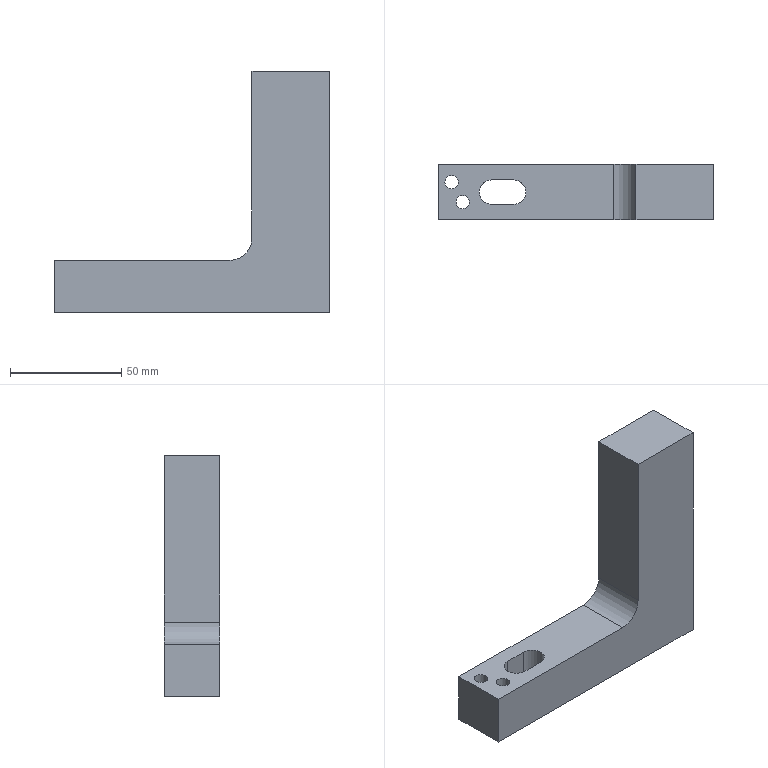Part | NX | features LIN_SOLID_COLOR 2 | 1 solid | 19 faces | box 124 x 25 x 108.5 mm | volume 139672 mm3 | plane 10 | cylinder 7 | cone 2 | commonest cylinder face diameters 6.001 x2 6.8 x2 11 x2 20 x1
STEP:
#1=CARTESIAN_POINT('',(938.,-125.5,49.4));
#2=VERTEX_POINT('',#1);
#3=CARTESIAN_POINT('',(938.,-125.5,46.));
#4=DIRECTION('',(-1.,0.,0.));
#5=DIRECTION('',(0.,0.,1.));
#6=AXIS2_PLACEMENT_3D('',#3,#4,#5);
#7=CIRCLE('',#6,3.4);
#8=EDGE_CURVE('',#2,#2,#7,.T.);
#9=ORIENTED_EDGE('',*,*,#8,.T.);
#10=EDGE_LOOP('',(#9));
#11=FACE_BOUND('',#10,.T.);
#12=CARTESIAN_POINT('',(938.,-138.,-46.5));
#13=VERTEX_POINT('',#12);
#14=CARTESIAN_POINT('',(938.,-113.,-46.5));
#15=VERTEX_POINT('',#14);
#16=CARTESIAN_POINT('',(938.,-43.,-46.5));
#17=DIRECTION('',(0.,-1.,0.));
#18=VECTOR('',#17,1000.);
#19=LINE('',#16,#18);
#20=EDGE_CURVE('',#13,#15,#19,.F.);
#21=ORIENTED_EDGE('',*,*,#20,.T.);
#22=CARTESIAN_POINT('',(938.,-113.,62.));
#23=VERTEX_POINT('',#22);
#24=CARTESIAN_POINT('',(938.,-113.,-16.051));
#25=DIRECTION('',(0.,0.,-1.));
#26=VECTOR('',#25,1000.);
#27=LINE('',#24,#26);
#28=EDGE_CURVE('',#15,#23,#27,.F.);
#29=ORIENTED_EDGE('',*,*,#28,.T.);
#30=CARTESIAN_POINT('',(938.,-138.,62.));
#31=VERTEX_POINT('',#30);
#32=CARTESIAN_POINT('',(938.,-128.,62.));
#33=DIRECTION('',(0.,-1.,0.));
#34=VECTOR('',#33,1000.);
#35=LINE('',#32,#34);
#36=EDGE_CURVE('',#31,#23,#35,.F.);
#37=ORIENTED_EDGE('',*,*,#36,.F.);
#38=CARTESIAN_POINT('',(938.,-138.,-16.5));
#39=DIRECTION('',(0.,0.,-1.));
#40=VECTOR('',#39,1000.);
#41=LINE('',#38,#40);
#42=EDGE_CURVE('',#13,#31,#41,.F.);
#43=ORIENTED_EDGE('',*,*,#42,.F.);
#44=EDGE_LOOP('',(#21,#29,#37,#43));
#45=FACE_BOUND('',#44,.T.);
#46=CARTESIAN_POINT('',(938.,-125.5,20.4));
#47=VERTEX_POINT('',#46);
#48=CARTESIAN_POINT('',(938.,-125.5,17.));
#49=DIRECTION('',(-1.,0.,0.));
#50=DIRECTION('',(0.,0.,1.));
#51=AXIS2_PLACEMENT_3D('',#48,#49,#50);
#52=CIRCLE('',#51,3.4);
#53=EDGE_CURVE('',#47,#47,#52,.T.);
#54=ORIENTED_EDGE('',*,*,#53,.T.);
#55=EDGE_LOOP('',(#54));
#56=FACE_BOUND('',#55,.T.);
#57=CARTESIAN_POINT('',(938.,-43.,-16.051));
#58=DIRECTION('',(-1.,0.,0.));
#59=DIRECTION('',(0.,0.,-1.));
#60=AXIS2_PLACEMENT_3D('',#57,#58,#59);
#61=PLANE('',#60);
#62=ADVANCED_FACE('',(#11,#45,#56),#61,.F.);
#63=CARTESIAN_POINT('',(814.,-138.,-23.));
#64=VERTEX_POINT('',#63);
#65=CARTESIAN_POINT('',(814.,-113.,-23.));
#66=VERTEX_POINT('',#65);
#67=CARTESIAN_POINT('',(814.,-128.,-23.));
#68=DIRECTION('',(0.,1.,0.));
#69=VECTOR('',#68,1000.);
#70=LINE('',#67,#69);
#71=EDGE_CURVE('',#64,#66,#70,.T.);
#72=ORIENTED_EDGE('',*,*,#71,.T.);
#73=CARTESIAN_POINT('',(814.,-113.,-46.5));
#74=VERTEX_POINT('',#73);
#75=CARTESIAN_POINT('',(814.,-113.,-16.5));
#76=DIRECTION('',(0.,0.,-1.));
#77=VECTOR('',#76,1000.);
#78=LINE('',#75,#77);
#79=EDGE_CURVE('',#66,#74,#78,.T.);
#80=ORIENTED_EDGE('',*,*,#79,.T.);
#81=CARTESIAN_POINT('',(814.,-138.,-46.5));
#82=VERTEX_POINT('',#81);
#83=CARTESIAN_POINT('',(814.,-128.,-46.5));
#84=DIRECTION('',(0.,-1.,0.));
#85=VECTOR('',#84,1000.);
#86=LINE('',#83,#85);
#87=EDGE_CURVE('',#74,#82,#86,.T.);
#88=ORIENTED_EDGE('',*,*,#87,.T.);
#89=CARTESIAN_POINT('',(814.,-138.,-16.5));
#90=DIRECTION('',(0.,0.,-1.));
#91=VECTOR('',#90,1000.);
#92=LINE('',#89,#91);
#93=EDGE_CURVE('',#64,#82,#92,.T.);
#94=ORIENTED_EDGE('',*,*,#93,.F.);
#95=EDGE_LOOP('',(#72,#80,#88,#94));
#96=FACE_BOUND('',#95,.T.);
#97=CARTESIAN_POINT('',(814.,-128.,-16.5));
#98=DIRECTION('',(-1.,0.,0.));
#99=DIRECTION('',(0.,0.,-1.));
#100=AXIS2_PLACEMENT_3D('',#97,#98,#99);
#101=PLANE('',#100);
#102=ADVANCED_FACE('',(#96),#101,.T.);
#103=CARTESIAN_POINT('',(848.,-131.,-23.));
#104=VERTEX_POINT('',#103);
#105=CARTESIAN_POINT('',(848.,-120.,-23.));
#106=VERTEX_POINT('',#105);
#107=CARTESIAN_POINT('',(848.,-125.5,-23.));
#108=DIRECTION('',(0.,0.,1.));
#109=DIRECTION('',(-1.,0.,0.));
#110=AXIS2_PLACEMENT_3D('',#107,#108,#109);
#111=CIRCLE('',#110,5.5);
#112=EDGE_CURVE('',#104,#106,#111,.T.);
#113=ORIENTED_EDGE('',*,*,#112,.T.);
#114=CARTESIAN_POINT('',(848.,-120.,-46.5));
#115=VERTEX_POINT('',#114);
#116=CARTESIAN_POINT('',(848.,-120.,-16.499));
#117=DIRECTION('',(0.,0.,-1.));
#118=VECTOR('',#117,1000.);
#119=LINE('',#116,#118);
#120=EDGE_CURVE('',#106,#115,#119,.T.);
#121=ORIENTED_EDGE('',*,*,#120,.T.);
#122=CARTESIAN_POINT('',(848.,-131.,-46.5));
#123=VERTEX_POINT('',#122);
#124=CARTESIAN_POINT('',(848.,-125.5,-46.5));
#125=DIRECTION('',(0.,0.,-1.));
#126=DIRECTION('',(1.,0.,0.));
#127=AXIS2_PLACEMENT_3D('',#124,#125,#126);
#128=CIRCLE('',#127,5.5);
#129=EDGE_CURVE('',#115,#123,#128,.T.);
#130=ORIENTED_EDGE('',*,*,#129,.T.);
#131=CARTESIAN_POINT('',(848.,-131.,-16.499));
#132=DIRECTION('',(0.,0.,-1.));
#133=VECTOR('',#132,1000.);
#134=LINE('',#131,#133);
#135=EDGE_CURVE('',#123,#104,#134,.F.);
#136=ORIENTED_EDGE('',*,*,#135,.T.);
#137=EDGE_LOOP('',(#113,#121,#130,#136));
#138=FACE_BOUND('',#137,.T.);
#139=CARTESIAN_POINT('',(848.,-125.5,-16.499));
#140=DIRECTION('',(0.,0.,-1.));
#141=DIRECTION('',(1.,0.,0.));
#142=AXIS2_PLACEMENT_3D('',#139,#140,#141);
#143=CYLINDRICAL_SURFACE('',#142,5.5);
#144=ADVANCED_FACE('',(#138),#143,.F.);
#145=CARTESIAN_POINT('',(838.,-131.,-46.5));
#146=VERTEX_POINT('',#145);
#147=CARTESIAN_POINT('',(843.,-131.,-46.5));
#148=DIRECTION('',(-1.,0.,0.));
#149=VECTOR('',#148,1000.);
#150=LINE('',#147,#149);
#151=EDGE_CURVE('',#123,#146,#150,.T.);
#152=ORIENTED_EDGE('',*,*,#151,.T.);
#153=CARTESIAN_POINT('',(838.,-131.,-23.));
#154=VERTEX_POINT('',#153);
#155=CARTESIAN_POINT('',(838.,-131.,-16.499));
#156=DIRECTION('',(0.,0.,-1.));
#157=VECTOR('',#156,1000.);
#158=LINE('',#155,#157);
#159=EDGE_CURVE('',#154,#146,#158,.T.);
#160=ORIENTED_EDGE('',*,*,#159,.F.);
#161=CARTESIAN_POINT('',(843.,-131.,-23.));
#162=DIRECTION('',(1.,0.,0.));
#163=VECTOR('',#162,1000.);
#164=LINE('',#161,#163);
#165=EDGE_CURVE('',#154,#104,#164,.T.);
#166=ORIENTED_EDGE('',*,*,#165,.T.);
#167=ORIENTED_EDGE('',*,*,#135,.F.);
#168=EDGE_LOOP('',(#152,#160,#166,#167));
#169=FACE_BOUND('',#168,.T.);
#170=CARTESIAN_POINT('',(838.,-131.,-16.499));
#171=DIRECTION('',(0.,-1.,0.));
#172=DIRECTION('',(0.,0.,-1.));
#173=AXIS2_PLACEMENT_3D('',#170,#171,#172);
#174=PLANE('',#173);
#175=ADVANCED_FACE('',(#169),#174,.F.);
#176=CARTESIAN_POINT('',(838.,-120.,-46.5));
#177=VERTEX_POINT('',#176);
#178=CARTESIAN_POINT('',(838.,-125.5,-46.5));
#179=DIRECTION('',(0.,0.,-1.));
#180=DIRECTION('',(1.,0.,0.));
#181=AXIS2_PLACEMENT_3D('',#178,#179,#180);
#182=CIRCLE('',#181,5.5);
#183=EDGE_CURVE('',#146,#177,#182,.T.);
#184=ORIENTED_EDGE('',*,*,#183,.T.);
#185=CARTESIAN_POINT('',(838.,-120.,-23.));
#186=VERTEX_POINT('',#185);
#187=CARTESIAN_POINT('',(838.,-120.,-16.499));
#188=DIRECTION('',(0.,0.,-1.));
#189=VECTOR('',#188,1000.);
#190=LINE('',#187,#189);
#191=EDGE_CURVE('',#177,#186,#190,.F.);
#192=ORIENTED_EDGE('',*,*,#191,.T.);
#193=CARTESIAN_POINT('',(838.,-125.5,-23.));
#194=DIRECTION('',(0.,0.,1.));
#195=DIRECTION('',(-1.,0.,0.));
#196=AXIS2_PLACEMENT_3D('',#193,#194,#195);
#197=CIRCLE('',#196,5.5);
#198=EDGE_CURVE('',#186,#154,#197,.T.);
#199=ORIENTED_EDGE('',*,*,#198,.T.);
#200=ORIENTED_EDGE('',*,*,#159,.T.);
#201=EDGE_LOOP('',(#184,#192,#199,#200));
#202=FACE_BOUND('',#201,.T.);
#203=CARTESIAN_POINT('',(838.,-125.5,-16.499));
#204=DIRECTION('',(0.,0.,-1.));
#205=DIRECTION('',(1.,0.,0.));
#206=AXIS2_PLACEMENT_3D('',#203,#204,#205);
#207=CYLINDRICAL_SURFACE('',#206,5.5);
#208=ADVANCED_FACE('',(#202),#207,.F.);
#209=CARTESIAN_POINT('',(843.,-120.,-46.5));
#210=DIRECTION('',(1.,0.,0.));
#211=VECTOR('',#210,1000.);
#212=LINE('',#209,#211);
#213=EDGE_CURVE('',#177,#115,#212,.T.);
#214=ORIENTED_EDGE('',*,*,#213,.T.);
#215=ORIENTED_EDGE('',*,*,#120,.F.);
#216=CARTESIAN_POINT('',(843.,-120.,-23.));
#217=DIRECTION('',(-1.,0.,0.));
#218=VECTOR('',#217,1000.);
#219=LINE('',#216,#218);
#220=EDGE_CURVE('',#106,#186,#219,.T.);
#221=ORIENTED_EDGE('',*,*,#220,.T.);
#222=ORIENTED_EDGE('',*,*,#191,.F.);
#223=EDGE_LOOP('',(#214,#215,#221,#222));
#224=FACE_BOUND('',#223,.T.);
#225=CARTESIAN_POINT('',(848.,-120.,-16.499));
#226=DIRECTION('',(0.,1.,0.));
#227=DIRECTION('',(0.,0.,1.));
#228=AXIS2_PLACEMENT_3D('',#225,#226,#227);
#229=PLANE('',#228);
#230=ADVANCED_FACE('',(#224),#229,.F.);
#231=CARTESIAN_POINT('',(816.999,-121.,-46.5));
#232=VERTEX_POINT('',#231);
#233=CARTESIAN_POINT('',(820.,-121.,-46.5));
#234=DIRECTION('',(0.,0.,-1.));
#235=DIRECTION('',(-1.,0.,0.));
#236=AXIS2_PLACEMENT_3D('',#233,#234,#235);
#237=CIRCLE('',#236,3.001);
#238=EDGE_CURVE('',#232,#232,#237,.T.);
#239=ORIENTED_EDGE('',*,*,#238,.T.);
#240=EDGE_LOOP('',(#239));
#241=FACE_BOUND('',#240,.T.);
#242=CARTESIAN_POINT('',(823.,-121.,-23.));
#243=VERTEX_POINT('',#242);
#244=CARTESIAN_POINT('',(820.,-121.,-23.));
#245=DIRECTION('',(0.,0.,1.));
#246=DIRECTION('',(1.,0.,0.));
#247=AXIS2_PLACEMENT_3D('',#244,#245,#246);
#248=CIRCLE('',#247,3.001);
#249=EDGE_CURVE('',#243,#243,#248,.T.);
#250=ORIENTED_EDGE('',*,*,#249,.T.);
#251=EDGE_LOOP('',(#250));
#252=FACE_BOUND('',#251,.T.);
#253=CARTESIAN_POINT('',(820.,-121.,-16.499));
#254=DIRECTION('',(0.,0.,-1.));
#255=DIRECTION('',(1.,0.,0.));
#256=AXIS2_PLACEMENT_3D('',#253,#254,#255);
#257=CYLINDRICAL_SURFACE('',#256,3.001);
#258=ADVANCED_FACE('',(#241,#252),#257,.F.);
#259=CARTESIAN_POINT('',(821.999,-130.,-46.5));
#260=VERTEX_POINT('',#259);
#261=CARTESIAN_POINT('',(825.,-130.,-46.5));
#262=DIRECTION('',(0.,0.,-1.));
#263=DIRECTION('',(-1.,0.,0.));
#264=AXIS2_PLACEMENT_3D('',#261,#262,#263);
#265=CIRCLE('',#264,3.001);
#266=EDGE_CURVE('',#260,#260,#265,.T.);
#267=ORIENTED_EDGE('',*,*,#266,.T.);
#268=EDGE_LOOP('',(#267));
#269=FACE_BOUND('',#268,.T.);
#270=CARTESIAN_POINT('',(828.,-130.,-23.));
#271=VERTEX_POINT('',#270);
#272=CARTESIAN_POINT('',(825.,-130.,-23.));
#273=DIRECTION('',(0.,0.,1.));
#274=DIRECTION('',(1.,0.,0.));
#275=AXIS2_PLACEMENT_3D('',#272,#273,#274);
#276=CIRCLE('',#275,3.001);
#277=EDGE_CURVE('',#271,#271,#276,.T.);
#278=ORIENTED_EDGE('',*,*,#277,.T.);
#279=EDGE_LOOP('',(#278));
#280=FACE_BOUND('',#279,.T.);
#281=CARTESIAN_POINT('',(825.,-130.,-16.499));
#282=DIRECTION('',(0.,0.,-1.));
#283=DIRECTION('',(1.,0.,0.));
#284=AXIS2_PLACEMENT_3D('',#281,#282,#283);
#285=CYLINDRICAL_SURFACE('',#284,3.001);
#286=ADVANCED_FACE('',(#269,#280),#285,.F.);
#287=ORIENTED_EDGE('',*,*,#266,.F.);
#288=EDGE_LOOP('',(#287));
#289=FACE_BOUND('',#288,.T.);
#290=ORIENTED_EDGE('',*,*,#238,.F.);
#291=EDGE_LOOP('',(#290));
#292=FACE_BOUND('',#291,.T.);
#293=ORIENTED_EDGE('',*,*,#213,.F.);
#294=ORIENTED_EDGE('',*,*,#183,.F.);
#295=ORIENTED_EDGE('',*,*,#151,.F.);
#296=ORIENTED_EDGE('',*,*,#129,.F.);
#297=EDGE_LOOP('',(#293,#294,#295,#296));
#298=FACE_BOUND('',#297,.T.);
#299=CARTESIAN_POINT('',(904.,-113.,-46.5));
#300=DIRECTION('',(-1.,0.,0.));
#301=VECTOR('',#300,1000.);
#302=LINE('',#299,#301);
#303=EDGE_CURVE('',#15,#74,#302,.T.);
#304=ORIENTED_EDGE('',*,*,#303,.F.);
#305=ORIENTED_EDGE('',*,*,#20,.F.);
#306=CARTESIAN_POINT('',(904.,-138.,-46.5));
#307=DIRECTION('',(1.,0.,0.));
#308=VECTOR('',#307,1000.);
#309=LINE('',#306,#308);
#310=EDGE_CURVE('',#82,#13,#309,.T.);
#311=ORIENTED_EDGE('',*,*,#310,.F.);
#312=ORIENTED_EDGE('',*,*,#87,.F.);
#313=EDGE_LOOP('',(#304,#305,#311,#312));
#314=FACE_BOUND('',#313,.T.);
#315=CARTESIAN_POINT('',(904.,-128.,-46.5));
#316=DIRECTION('',(0.,0.,-1.));
#317=DIRECTION('',(1.,0.,0.));
#318=AXIS2_PLACEMENT_3D('',#315,#316,#317);
#319=PLANE('',#318);
#320=ADVANCED_FACE('',(#289,#292,#298,#314),#319,.T.);
#321=ORIENTED_EDGE('',*,*,#310,.T.);
#322=ORIENTED_EDGE('',*,*,#42,.T.);
#323=CARTESIAN_POINT('',(903.,-138.,62.));
#324=VERTEX_POINT('',#323);
#325=CARTESIAN_POINT('',(904.,-138.,62.));
#326=DIRECTION('',(-1.,0.,0.));
#327=VECTOR('',#326,1000.);
#328=LINE('',#325,#327);
#329=EDGE_CURVE('',#31,#324,#328,.T.);
#330=ORIENTED_EDGE('',*,*,#329,.T.);
#331=CARTESIAN_POINT('',(903.,-138.,-13.));
#332=VERTEX_POINT('',#331);
#333=CARTESIAN_POINT('',(903.,-138.,-34.75));
#334=DIRECTION('',(0.,0.,-1.));
#335=VECTOR('',#334,1000.);
#336=LINE('',#333,#335);
#337=EDGE_CURVE('',#324,#332,#336,.T.);
#338=ORIENTED_EDGE('',*,*,#337,.T.);
#339=CARTESIAN_POINT('',(893.,-138.,-23.));
#340=VERTEX_POINT('',#339);
#341=CARTESIAN_POINT('',(893.,-138.,-13.));
#342=DIRECTION('',(0.,-1.,0.));
#343=DIRECTION('',(0.,0.,-1.));
#344=AXIS2_PLACEMENT_3D('',#341,#342,#343);
#345=CIRCLE('',#344,10.);
#346=EDGE_CURVE('',#332,#340,#345,.F.);
#347=ORIENTED_EDGE('',*,*,#346,.T.);
#348=CARTESIAN_POINT('',(904.,-138.,-23.));
#349=DIRECTION('',(-1.,0.,0.));
#350=VECTOR('',#349,1000.);
#351=LINE('',#348,#350);
#352=EDGE_CURVE('',#340,#64,#351,.T.);
#353=ORIENTED_EDGE('',*,*,#352,.T.);
#354=ORIENTED_EDGE('',*,*,#93,.T.);
#355=EDGE_LOOP('',(#321,#322,#330,#338,#347,#353,#354));
#356=FACE_BOUND('',#355,.T.);
#357=CARTESIAN_POINT('',(904.,-138.,-16.5));
#358=DIRECTION('',(0.,-1.,0.));
#359=DIRECTION('',(0.,0.,-1.));
#360=AXIS2_PLACEMENT_3D('',#357,#358,#359);
#361=PLANE('',#360);
#362=ADVANCED_FACE('',(#356),#361,.T.);
#363=CARTESIAN_POINT('',(893.,-113.,-23.));
#364=VERTEX_POINT('',#363);
#365=CARTESIAN_POINT('',(904.,-113.,-23.));
#366=DIRECTION('',(1.,0.,0.));
#367=VECTOR('',#366,1000.);
#368=LINE('',#365,#367);
#369=EDGE_CURVE('',#66,#364,#368,.T.);
#370=ORIENTED_EDGE('',*,*,#369,.T.);
#371=CARTESIAN_POINT('',(903.,-113.,-13.));
#372=VERTEX_POINT('',#371);
#373=CARTESIAN_POINT('',(893.,-113.,-13.));
#374=DIRECTION('',(0.,1.,0.));
#375=DIRECTION('',(0.,0.,1.));
#376=AXIS2_PLACEMENT_3D('',#373,#374,#375);
#377=CIRCLE('',#376,10.);
#378=EDGE_CURVE('',#364,#372,#377,.F.);
#379=ORIENTED_EDGE('',*,*,#378,.T.);
#380=CARTESIAN_POINT('',(903.,-113.,62.));
#381=VERTEX_POINT('',#380);
#382=CARTESIAN_POINT('',(903.,-113.,-16.5));
#383=DIRECTION('',(0.,0.,-1.));
#384=VECTOR('',#383,1000.);
#385=LINE('',#382,#384);
#386=EDGE_CURVE('',#381,#372,#385,.T.);
#387=ORIENTED_EDGE('',*,*,#386,.F.);
#388=CARTESIAN_POINT('',(904.,-113.,62.));
#389=DIRECTION('',(1.,0.,0.));
#390=VECTOR('',#389,1000.);
#391=LINE('',#388,#390);
#392=EDGE_CURVE('',#381,#23,#391,.T.);
#393=ORIENTED_EDGE('',*,*,#392,.T.);
#394=ORIENTED_EDGE('',*,*,#28,.F.);
#395=ORIENTED_EDGE('',*,*,#303,.T.);
#396=ORIENTED_EDGE('',*,*,#79,.F.);
#397=EDGE_LOOP('',(#370,#379,#387,#393,#394,#395,#396));
#398=FACE_BOUND('',#397,.T.);
#399=CARTESIAN_POINT('',(904.,-113.,-16.5));
#400=DIRECTION('',(0.,1.,0.));
#401=DIRECTION('',(0.,0.,1.));
#402=AXIS2_PLACEMENT_3D('',#399,#400,#401);
#403=PLANE('',#402);
#404=ADVANCED_FACE('',(#398),#403,.T.);
#405=ORIENTED_EDGE('',*,*,#277,.F.);
#406=EDGE_LOOP('',(#405));
#407=FACE_BOUND('',#406,.T.);
#408=ORIENTED_EDGE('',*,*,#249,.F.);
#409=EDGE_LOOP('',(#408));
#410=FACE_BOUND('',#409,.T.);
#411=ORIENTED_EDGE('',*,*,#220,.F.);
#412=ORIENTED_EDGE('',*,*,#112,.F.);
#413=ORIENTED_EDGE('',*,*,#165,.F.);
#414=ORIENTED_EDGE('',*,*,#198,.F.);
#415=EDGE_LOOP('',(#411,#412,#413,#414));
#416=FACE_BOUND('',#415,.T.);
#417=ORIENTED_EDGE('',*,*,#352,.F.);
#418=CARTESIAN_POINT('',(893.,-128.,-23.));
#419=DIRECTION('',(0.,1.,0.));
#420=VECTOR('',#419,1000.);
#421=LINE('',#418,#420);
#422=EDGE_CURVE('',#340,#364,#421,.T.);
#423=ORIENTED_EDGE('',*,*,#422,.T.);
#424=ORIENTED_EDGE('',*,*,#369,.F.);
#425=ORIENTED_EDGE('',*,*,#71,.F.);
#426=EDGE_LOOP('',(#417,#423,#424,#425));
#427=FACE_BOUND('',#426,.T.);
#428=CARTESIAN_POINT('',(904.,-128.,-23.));
#429=DIRECTION('',(0.,0.,1.));
#430=DIRECTION('',(-1.,0.,0.));
#431=AXIS2_PLACEMENT_3D('',#428,#429,#430);
#432=PLANE('',#431);
#433=ADVANCED_FACE('',(#407,#410,#416,#427),#432,.T.);
#434=CARTESIAN_POINT('',(903.,-125.5,62.));
#435=DIRECTION('',(0.,-1.,0.));
#436=VECTOR('',#435,1000.);
#437=LINE('',#434,#436);
#438=EDGE_CURVE('',#381,#324,#437,.T.);
#439=ORIENTED_EDGE('',*,*,#438,.T.);
#440=ORIENTED_EDGE('',*,*,#329,.F.);
#441=ORIENTED_EDGE('',*,*,#36,.T.);
#442=ORIENTED_EDGE('',*,*,#392,.F.);
#443=EDGE_LOOP('',(#439,#440,#441,#442));
#444=FACE_BOUND('',#443,.T.);
#445=CARTESIAN_POINT('',(904.,-128.,62.));
#446=DIRECTION('',(0.,0.,1.));
#447=DIRECTION('',(-1.,0.,0.));
#448=AXIS2_PLACEMENT_3D('',#445,#446,#447);
#449=PLANE('',#448);
#450=ADVANCED_FACE('',(#444),#449,.T.);
#451=ORIENTED_EDGE('',*,*,#386,.T.);
#452=CARTESIAN_POINT('',(903.,-125.5,-13.));
#453=DIRECTION('',(0.,1.,0.));
#454=VECTOR('',#453,1000.);
#455=LINE('',#452,#454);
#456=EDGE_CURVE('',#372,#332,#455,.F.);
#457=ORIENTED_EDGE('',*,*,#456,.T.);
#458=ORIENTED_EDGE('',*,*,#337,.F.);
#459=ORIENTED_EDGE('',*,*,#438,.F.);
#460=EDGE_LOOP('',(#451,#457,#458,#459));
#461=FACE_BOUND('',#460,.T.);
#462=CARTESIAN_POINT('',(903.,-125.5,-34.75));
#463=DIRECTION('',(1.,0.,0.));
#464=DIRECTION('',(0.,0.,1.));
#465=AXIS2_PLACEMENT_3D('',#462,#463,#464);
#466=PLANE('',#465);
#467=ADVANCED_FACE('',(#461),#466,.F.);
#468=ORIENTED_EDGE('',*,*,#346,.F.);
#469=ORIENTED_EDGE('',*,*,#456,.F.);
#470=ORIENTED_EDGE('',*,*,#378,.F.);
#471=ORIENTED_EDGE('',*,*,#422,.F.);
#472=EDGE_LOOP('',(#468,#469,#470,#471));
#473=FACE_BOUND('',#472,.T.);
#474=CARTESIAN_POINT('',(893.,-128.,-13.));
#475=DIRECTION('',(0.,1.,0.));
#476=DIRECTION('',(0.,0.,1.));
#477=AXIS2_PLACEMENT_3D('',#474,#475,#476);
#478=CYLINDRICAL_SURFACE('',#477,10.);
#479=ADVANCED_FACE('',(#473),#478,.F.);
#480=CARTESIAN_POINT('',(912.4,-125.5,49.4));
#481=VERTEX_POINT('',#480);
#482=CARTESIAN_POINT('',(912.4,-125.5,46.));
#483=DIRECTION('',(-1.,0.,0.));
#484=DIRECTION('',(0.,0.,1.));
#485=AXIS2_PLACEMENT_3D('',#482,#483,#484);
#486=CIRCLE('',#485,3.4);
#487=EDGE_CURVE('',#481,#481,#486,.T.);
#488=ORIENTED_EDGE('',*,*,#487,.T.);
#489=EDGE_LOOP('',(#488));
#490=FACE_BOUND('',#489,.T.);
#491=ORIENTED_EDGE('',*,*,#8,.F.);
#492=EDGE_LOOP('',(#491));
#493=FACE_BOUND('',#492,.T.);
#494=CARTESIAN_POINT('',(938.,-125.5,46.));
#495=DIRECTION('',(-1.,0.,0.));
#496=DIRECTION('',(0.,0.,1.));
#497=AXIS2_PLACEMENT_3D('',#494,#495,#496);
#498=CYLINDRICAL_SURFACE('',#497,3.4);
#499=ADVANCED_FACE('',(#490,#493),#498,.F.);
#500=CARTESIAN_POINT('',(909.,-125.5,46.));
#501=VERTEX_POINT('',#500);
#502=VERTEX_LOOP('',#501);
#503=FACE_BOUND('',#502,.T.);
#504=ORIENTED_EDGE('',*,*,#487,.F.);
#505=EDGE_LOOP('',(#504));
#506=FACE_BOUND('',#505,.T.);
#507=CARTESIAN_POINT('',(912.4,-125.5,46.));
#508=DIRECTION('',(1.,0.,0.));
#509=DIRECTION('',(0.,0.,-1.));
#510=AXIS2_PLACEMENT_3D('',#507,#508,#509);
#511=CONICAL_SURFACE('',#510,3.4,0.7854);
#512=ADVANCED_FACE('',(#503,#506),#511,.F.);
#513=CARTESIAN_POINT('',(912.4,-125.5,20.4));
#514=VERTEX_POINT('',#513);
#515=CARTESIAN_POINT('',(912.4,-125.5,17.));
#516=DIRECTION('',(-1.,0.,0.));
#517=DIRECTION('',(0.,0.,1.));
#518=AXIS2_PLACEMENT_3D('',#515,#516,#517);
#519=CIRCLE('',#518,3.4);
#520=EDGE_CURVE('',#514,#514,#519,.T.);
#521=ORIENTED_EDGE('',*,*,#520,.T.);
#522=EDGE_LOOP('',(#521));
#523=FACE_BOUND('',#522,.T.);
#524=ORIENTED_EDGE('',*,*,#53,.F.);
#525=EDGE_LOOP('',(#524));
#526=FACE_BOUND('',#525,.T.);
#527=CARTESIAN_POINT('',(938.,-125.5,17.));
#528=DIRECTION('',(-1.,0.,0.));
#529=DIRECTION('',(0.,0.,1.));
#530=AXIS2_PLACEMENT_3D('',#527,#528,#529);
#531=CYLINDRICAL_SURFACE('',#530,3.4);
#532=ADVANCED_FACE('',(#523,#526),#531,.F.);
#533=CARTESIAN_POINT('',(909.,-125.5,17.));
#534=VERTEX_POINT('',#533);
#535=VERTEX_LOOP('',#534);
#536=FACE_BOUND('',#535,.T.);
#537=ORIENTED_EDGE('',*,*,#520,.F.);
#538=EDGE_LOOP('',(#537));
#539=FACE_BOUND('',#538,.T.);
#540=CARTESIAN_POINT('',(912.4,-125.5,17.));
#541=DIRECTION('',(1.,0.,0.));
#542=DIRECTION('',(0.,0.,-1.));
#543=AXIS2_PLACEMENT_3D('',#540,#541,#542);
#544=CONICAL_SURFACE('',#543,3.4,0.7854);
#545=ADVANCED_FACE('',(#536,#539),#544,.F.);
#546=CLOSED_SHELL('',(#62,#102,#144,#175,#208,#230,#258,#286,#320,#362,#404,#433,#450,#467,#479,#499,#512,#532,#545));
#547=MANIFOLD_SOLID_BREP('',#546);
#548=(LENGTH_UNIT()NAMED_UNIT(*)SI_UNIT(.MILLI.,.METRE.));
#549=UNCERTAINTY_MEASURE_WITH_UNIT(LENGTH_MEASURE(0.00001),#548,'','');
#550=(NAMED_UNIT(*)PLANE_ANGLE_UNIT()SI_UNIT($,.RADIAN.));
#551=(NAMED_UNIT(*)SI_UNIT($,.STERADIAN.)SOLID_ANGLE_UNIT());
#552=(GEOMETRIC_REPRESENTATION_CONTEXT(3)GLOBAL_UNCERTAINTY_ASSIGNED_CONTEXT((#549))GLOBAL_UNIT_ASSIGNED_CONTEXT((#548,#550,#551))REPRESENTATION_CONTEXT('',''));
#553=ADVANCED_BREP_SHAPE_REPRESENTATION('',(#547),#552);